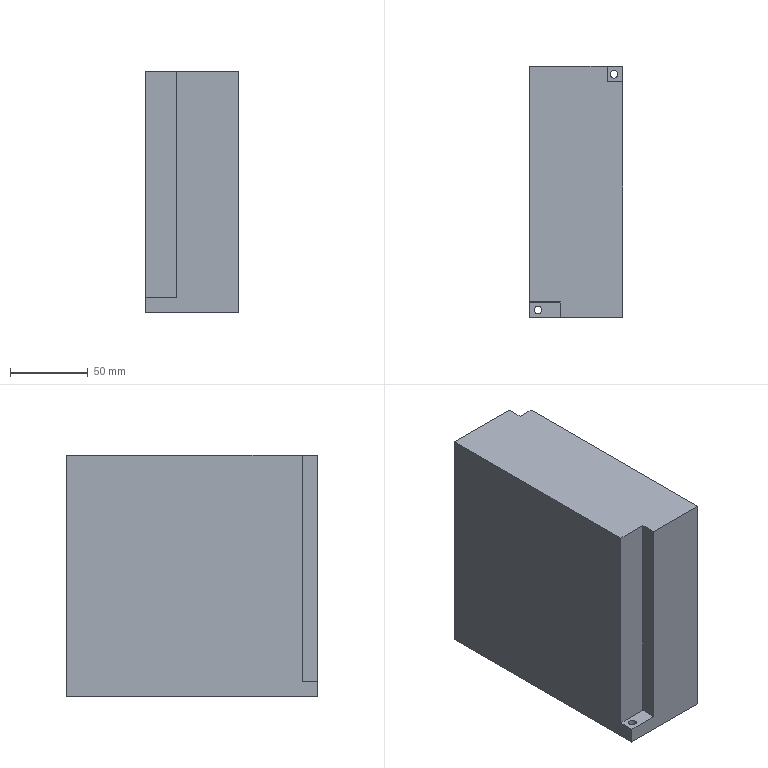Part | SolidWorks | features Cut 2, Extrusion 1 | 1 solid | 16 faces | box 60.2 x 162 x 155.9 mm | volume 1476236 mm3 | plane 12 | cylinder 4 | commonest cylinder face diameters 5 x4
STEP:
#1=CARTESIAN_POINT('',(-27.,-76.,0.));
#2=VERTEX_POINT('',#1);
#3=CARTESIAN_POINT('',(-22.,-76.,0.));
#4=VERTEX_POINT('',#3);
#5=CARTESIAN_POINT('',(-24.5,-76.,0.));
#6=DIRECTION('',(0.,0.,1.));
#7=DIRECTION('',(1.,0.,0.));
#8=AXIS2_PLACEMENT_3D('',#5,#6,#7);
#9=CIRCLE('',#8,2.5);
#10=EDGE_CURVE('',#2,#4,#9,.T.);
#11=ORIENTED_EDGE('',*,*,#10,.F.);
#12=CARTESIAN_POINT('',(-27.,-76.,10.));
#13=VERTEX_POINT('',#12);
#14=CARTESIAN_POINT('',(-27.,-76.,0.));
#15=DIRECTION('',(0.,0.,1.));
#16=VECTOR('',#15,1000.);
#17=LINE('',#14,#16);
#18=EDGE_CURVE('',#2,#13,#17,.T.);
#19=ORIENTED_EDGE('',*,*,#18,.T.);
#20=CARTESIAN_POINT('',(-22.,-76.,10.));
#21=VERTEX_POINT('',#20);
#22=CARTESIAN_POINT('',(-24.5,-76.,10.));
#23=DIRECTION('',(0.,0.,-1.));
#24=DIRECTION('',(-1.,0.,0.));
#25=AXIS2_PLACEMENT_3D('',#22,#23,#24);
#26=CIRCLE('',#25,2.5);
#27=EDGE_CURVE('',#21,#13,#26,.T.);
#28=ORIENTED_EDGE('',*,*,#27,.F.);
#29=CARTESIAN_POINT('',(-22.,-76.,0.));
#30=DIRECTION('',(0.,0.,1.));
#31=VECTOR('',#30,1000.);
#32=LINE('',#29,#31);
#33=EDGE_CURVE('',#4,#21,#32,.T.);
#34=ORIENTED_EDGE('',*,*,#33,.F.);
#35=EDGE_LOOP('',(#11,#19,#28,#34));
#36=FACE_OUTER_BOUND('',#35,.T.);
#37=CARTESIAN_POINT('',(-24.5,-76.,0.));
#38=DIRECTION('',(0.,0.,1.));
#39=DIRECTION('',(1.,0.,0.));
#40=AXIS2_PLACEMENT_3D('',#37,#38,#39);
#41=CYLINDRICAL_SURFACE('',#40,2.5);
#42=ADVANCED_FACE('',(#36),#41,.F.);
#43=CARTESIAN_POINT('',(22.,76.,0.));
#44=VERTEX_POINT('',#43);
#45=CARTESIAN_POINT('',(27.,76.,0.));
#46=VERTEX_POINT('',#45);
#47=CARTESIAN_POINT('',(24.5,76.,0.));
#48=DIRECTION('',(0.,0.,1.));
#49=DIRECTION('',(1.,0.,0.));
#50=AXIS2_PLACEMENT_3D('',#47,#48,#49);
#51=CIRCLE('',#50,2.5);
#52=EDGE_CURVE('',#44,#46,#51,.T.);
#53=ORIENTED_EDGE('',*,*,#52,.F.);
#54=CARTESIAN_POINT('',(22.,76.,10.));
#55=VERTEX_POINT('',#54);
#56=CARTESIAN_POINT('',(22.,76.,0.));
#57=DIRECTION('',(0.,0.,1.));
#58=VECTOR('',#57,1000.);
#59=LINE('',#56,#58);
#60=EDGE_CURVE('',#44,#55,#59,.T.);
#61=ORIENTED_EDGE('',*,*,#60,.T.);
#62=CARTESIAN_POINT('',(27.,76.,10.));
#63=VERTEX_POINT('',#62);
#64=CARTESIAN_POINT('',(24.5,76.,10.));
#65=DIRECTION('',(0.,0.,-1.));
#66=DIRECTION('',(-1.,0.,0.));
#67=AXIS2_PLACEMENT_3D('',#64,#65,#66);
#68=CIRCLE('',#67,2.5);
#69=EDGE_CURVE('',#63,#55,#68,.T.);
#70=ORIENTED_EDGE('',*,*,#69,.F.);
#71=CARTESIAN_POINT('',(27.,76.,0.));
#72=DIRECTION('',(0.,0.,1.));
#73=VECTOR('',#72,1000.);
#74=LINE('',#71,#73);
#75=EDGE_CURVE('',#46,#63,#74,.T.);
#76=ORIENTED_EDGE('',*,*,#75,.F.);
#77=EDGE_LOOP('',(#53,#61,#70,#76));
#78=FACE_OUTER_BOUND('',#77,.T.);
#79=CARTESIAN_POINT('',(24.5,76.,0.));
#80=DIRECTION('',(0.,0.,1.));
#81=DIRECTION('',(1.,0.,0.));
#82=AXIS2_PLACEMENT_3D('',#79,#80,#81);
#83=CYLINDRICAL_SURFACE('',#82,2.5);
#84=ADVANCED_FACE('',(#78),#83,.F.);
#85=CARTESIAN_POINT('',(-30.1,-71.,10.));
#86=VERTEX_POINT('',#85);
#87=CARTESIAN_POINT('',(-30.1,-81.,10.));
#88=VERTEX_POINT('',#87);
#89=CARTESIAN_POINT('',(-30.1,-81.,10.));
#90=DIRECTION('',(0.,-1.,0.));
#91=VECTOR('',#90,1000.);
#92=LINE('',#89,#91);
#93=EDGE_CURVE('',#86,#88,#92,.T.);
#94=ORIENTED_EDGE('',*,*,#93,.F.);
#95=CARTESIAN_POINT('',(-30.1,-71.,155.9));
#96=VERTEX_POINT('',#95);
#97=CARTESIAN_POINT('',(-30.1,-71.,10.));
#98=DIRECTION('',(0.,0.,1.));
#99=VECTOR('',#98,1000.);
#100=LINE('',#97,#99);
#101=EDGE_CURVE('',#86,#96,#100,.T.);
#102=ORIENTED_EDGE('',*,*,#101,.T.);
#103=CARTESIAN_POINT('',(-30.1,81.,155.9));
#104=VERTEX_POINT('',#103);
#105=CARTESIAN_POINT('',(-30.1,81.,155.9));
#106=DIRECTION('',(0.,-1.,0.));
#107=VECTOR('',#106,1000.);
#108=LINE('',#105,#107);
#109=EDGE_CURVE('',#104,#96,#108,.T.);
#110=ORIENTED_EDGE('',*,*,#109,.F.);
#111=CARTESIAN_POINT('',(-30.1,81.,0.));
#112=VERTEX_POINT('',#111);
#113=CARTESIAN_POINT('',(-30.1,81.,155.9));
#114=DIRECTION('',(0.,0.,-1.));
#115=VECTOR('',#114,1000.);
#116=LINE('',#113,#115);
#117=EDGE_CURVE('',#104,#112,#116,.T.);
#118=ORIENTED_EDGE('',*,*,#117,.T.);
#119=CARTESIAN_POINT('',(-30.1,-81.,0.));
#120=VERTEX_POINT('',#119);
#121=CARTESIAN_POINT('',(-30.1,81.,0.));
#122=DIRECTION('',(0.,-1.,0.));
#123=VECTOR('',#122,1000.);
#124=LINE('',#121,#123);
#125=EDGE_CURVE('',#112,#120,#124,.T.);
#126=ORIENTED_EDGE('',*,*,#125,.T.);
#127=CARTESIAN_POINT('',(-30.1,-81.,155.9));
#128=DIRECTION('',(0.,0.,-1.));
#129=VECTOR('',#128,1000.);
#130=LINE('',#127,#129);
#131=EDGE_CURVE('',#88,#120,#130,.T.);
#132=ORIENTED_EDGE('',*,*,#131,.F.);
#133=EDGE_LOOP('',(#94,#102,#110,#118,#126,#132));
#134=FACE_OUTER_BOUND('',#133,.T.);
#135=CARTESIAN_POINT('',(-30.1,81.,155.9));
#136=DIRECTION('',(1.,0.,0.));
#137=DIRECTION('',(0.,1.,0.));
#138=AXIS2_PLACEMENT_3D('',#135,#136,#137);
#139=PLANE('',#138);
#140=ADVANCED_FACE('',(#134),#139,.F.);
#141=CARTESIAN_POINT('',(-10.1,-81.,155.9));
#142=VERTEX_POINT('',#141);
#143=CARTESIAN_POINT('',(30.1,-81.,155.9));
#144=VERTEX_POINT('',#143);
#145=CARTESIAN_POINT('',(-30.1,-81.,155.9));
#146=DIRECTION('',(1.,0.,0.));
#147=VECTOR('',#146,1000.);
#148=LINE('',#145,#147);
#149=EDGE_CURVE('',#142,#144,#148,.T.);
#150=ORIENTED_EDGE('',*,*,#149,.F.);
#151=CARTESIAN_POINT('',(-10.1,-81.,10.));
#152=VERTEX_POINT('',#151);
#153=CARTESIAN_POINT('',(-10.1,-81.,10.));
#154=DIRECTION('',(0.,0.,1.));
#155=VECTOR('',#154,1000.);
#156=LINE('',#153,#155);
#157=EDGE_CURVE('',#152,#142,#156,.T.);
#158=ORIENTED_EDGE('',*,*,#157,.F.);
#159=CARTESIAN_POINT('',(-30.1,-81.,10.));
#160=DIRECTION('',(1.,0.,0.));
#161=VECTOR('',#160,1000.);
#162=LINE('',#159,#161);
#163=EDGE_CURVE('',#88,#152,#162,.T.);
#164=ORIENTED_EDGE('',*,*,#163,.F.);
#165=ORIENTED_EDGE('',*,*,#131,.T.);
#166=CARTESIAN_POINT('',(30.1,-81.,0.));
#167=VERTEX_POINT('',#166);
#168=CARTESIAN_POINT('',(-30.1,-81.,0.));
#169=DIRECTION('',(1.,0.,0.));
#170=VECTOR('',#169,1000.);
#171=LINE('',#168,#170);
#172=EDGE_CURVE('',#120,#167,#171,.T.);
#173=ORIENTED_EDGE('',*,*,#172,.T.);
#174=CARTESIAN_POINT('',(30.1,-81.,155.9));
#175=DIRECTION('',(0.,0.,-1.));
#176=VECTOR('',#175,1000.);
#177=LINE('',#174,#176);
#178=EDGE_CURVE('',#144,#167,#177,.T.);
#179=ORIENTED_EDGE('',*,*,#178,.F.);
#180=EDGE_LOOP('',(#150,#158,#164,#165,#173,#179));
#181=FACE_OUTER_BOUND('',#180,.T.);
#182=CARTESIAN_POINT('',(-30.1,-81.,155.9));
#183=DIRECTION('',(0.,1.,0.));
#184=DIRECTION('',(0.,0.,1.));
#185=AXIS2_PLACEMENT_3D('',#182,#183,#184);
#186=PLANE('',#185);
#187=ADVANCED_FACE('',(#181),#186,.F.);
#188=CARTESIAN_POINT('',(30.1,71.,10.));
#189=VERTEX_POINT('',#188);
#190=CARTESIAN_POINT('',(30.1,81.,10.));
#191=VERTEX_POINT('',#190);
#192=CARTESIAN_POINT('',(30.1,81.,10.));
#193=DIRECTION('',(0.,1.,0.));
#194=VECTOR('',#193,1000.);
#195=LINE('',#192,#194);
#196=EDGE_CURVE('',#189,#191,#195,.T.);
#197=ORIENTED_EDGE('',*,*,#196,.F.);
#198=CARTESIAN_POINT('',(30.1,71.,155.9));
#199=VERTEX_POINT('',#198);
#200=CARTESIAN_POINT('',(30.1,71.,10.));
#201=DIRECTION('',(0.,0.,1.));
#202=VECTOR('',#201,1000.);
#203=LINE('',#200,#202);
#204=EDGE_CURVE('',#189,#199,#203,.T.);
#205=ORIENTED_EDGE('',*,*,#204,.T.);
#206=CARTESIAN_POINT('',(30.1,81.,155.9));
#207=DIRECTION('',(0.,1.,0.));
#208=VECTOR('',#207,1000.);
#209=LINE('',#206,#208);
#210=EDGE_CURVE('',#144,#199,#209,.T.);
#211=ORIENTED_EDGE('',*,*,#210,.F.);
#212=ORIENTED_EDGE('',*,*,#178,.T.);
#213=CARTESIAN_POINT('',(30.1,81.,0.));
#214=VERTEX_POINT('',#213);
#215=CARTESIAN_POINT('',(30.1,81.,0.));
#216=DIRECTION('',(0.,1.,0.));
#217=VECTOR('',#216,1000.);
#218=LINE('',#215,#217);
#219=EDGE_CURVE('',#167,#214,#218,.T.);
#220=ORIENTED_EDGE('',*,*,#219,.T.);
#221=CARTESIAN_POINT('',(30.1,81.,155.9));
#222=DIRECTION('',(0.,0.,-1.));
#223=VECTOR('',#222,1000.);
#224=LINE('',#221,#223);
#225=EDGE_CURVE('',#191,#214,#224,.T.);
#226=ORIENTED_EDGE('',*,*,#225,.F.);
#227=EDGE_LOOP('',(#197,#205,#211,#212,#220,#226));
#228=FACE_OUTER_BOUND('',#227,.T.);
#229=CARTESIAN_POINT('',(30.1,81.,155.9));
#230=DIRECTION('',(-1.,0.,0.));
#231=DIRECTION('',(0.,-1.,0.));
#232=AXIS2_PLACEMENT_3D('',#229,#230,#231);
#233=PLANE('',#232);
#234=ADVANCED_FACE('',(#228),#233,.F.);
#235=CARTESIAN_POINT('',(20.1,81.,155.9));
#236=VERTEX_POINT('',#235);
#237=CARTESIAN_POINT('',(-30.1,81.,155.9));
#238=DIRECTION('',(-1.,0.,0.));
#239=VECTOR('',#238,1000.);
#240=LINE('',#237,#239);
#241=EDGE_CURVE('',#236,#104,#240,.T.);
#242=ORIENTED_EDGE('',*,*,#241,.F.);
#243=CARTESIAN_POINT('',(20.1,81.,10.));
#244=VERTEX_POINT('',#243);
#245=CARTESIAN_POINT('',(20.1,81.,10.));
#246=DIRECTION('',(0.,0.,1.));
#247=VECTOR('',#246,1000.);
#248=LINE('',#245,#247);
#249=EDGE_CURVE('',#244,#236,#248,.T.);
#250=ORIENTED_EDGE('',*,*,#249,.F.);
#251=CARTESIAN_POINT('',(30.1,81.,10.));
#252=DIRECTION('',(-1.,0.,0.));
#253=VECTOR('',#252,1000.);
#254=LINE('',#251,#253);
#255=EDGE_CURVE('',#191,#244,#254,.T.);
#256=ORIENTED_EDGE('',*,*,#255,.F.);
#257=ORIENTED_EDGE('',*,*,#225,.T.);
#258=CARTESIAN_POINT('',(-30.1,81.,0.));
#259=DIRECTION('',(-1.,0.,0.));
#260=VECTOR('',#259,1000.);
#261=LINE('',#258,#260);
#262=EDGE_CURVE('',#214,#112,#261,.T.);
#263=ORIENTED_EDGE('',*,*,#262,.T.);
#264=ORIENTED_EDGE('',*,*,#117,.F.);
#265=EDGE_LOOP('',(#242,#250,#256,#257,#263,#264));
#266=FACE_OUTER_BOUND('',#265,.T.);
#267=CARTESIAN_POINT('',(-30.1,81.,155.9));
#268=DIRECTION('',(0.,-1.,0.));
#269=DIRECTION('',(0.,0.,-1.));
#270=AXIS2_PLACEMENT_3D('',#267,#268,#269);
#271=PLANE('',#270);
#272=ADVANCED_FACE('',(#266),#271,.F.);
#273=CARTESIAN_POINT('',(20.1,71.,155.9));
#274=VERTEX_POINT('',#273);
#275=CARTESIAN_POINT('',(30.1,71.,155.9));
#276=DIRECTION('',(1.,0.,0.));
#277=VECTOR('',#276,1000.);
#278=LINE('',#275,#277);
#279=EDGE_CURVE('',#274,#199,#278,.T.);
#280=ORIENTED_EDGE('',*,*,#279,.F.);
#281=CARTESIAN_POINT('',(20.1,81.,155.9));
#282=DIRECTION('',(0.,-1.,0.));
#283=VECTOR('',#282,1000.);
#284=LINE('',#281,#283);
#285=EDGE_CURVE('',#236,#274,#284,.T.);
#286=ORIENTED_EDGE('',*,*,#285,.F.);
#287=ORIENTED_EDGE('',*,*,#241,.T.);
#288=ORIENTED_EDGE('',*,*,#109,.T.);
#289=CARTESIAN_POINT('',(-10.1,-71.,155.9));
#290=VERTEX_POINT('',#289);
#291=CARTESIAN_POINT('',(-30.1,-71.,155.9));
#292=DIRECTION('',(-1.,0.,0.));
#293=VECTOR('',#292,1000.);
#294=LINE('',#291,#293);
#295=EDGE_CURVE('',#290,#96,#294,.T.);
#296=ORIENTED_EDGE('',*,*,#295,.F.);
#297=CARTESIAN_POINT('',(-10.1,-81.,155.9));
#298=DIRECTION('',(0.,1.,0.));
#299=VECTOR('',#298,1000.);
#300=LINE('',#297,#299);
#301=EDGE_CURVE('',#142,#290,#300,.T.);
#302=ORIENTED_EDGE('',*,*,#301,.F.);
#303=ORIENTED_EDGE('',*,*,#149,.T.);
#304=ORIENTED_EDGE('',*,*,#210,.T.);
#305=EDGE_LOOP('',(#280,#286,#287,#288,#296,#302,#303,#304));
#306=FACE_OUTER_BOUND('',#305,.T.);
#307=CARTESIAN_POINT('',(-30.1,-81.,155.9));
#308=DIRECTION('',(0.,0.,1.));
#309=DIRECTION('',(1.,0.,0.));
#310=AXIS2_PLACEMENT_3D('',#307,#308,#309);
#311=PLANE('',#310);
#312=ADVANCED_FACE('',(#306),#311,.T.);
#313=CARTESIAN_POINT('',(-24.5,-76.,0.));
#314=DIRECTION('',(0.,0.,1.));
#315=DIRECTION('',(1.,0.,0.));
#316=AXIS2_PLACEMENT_3D('',#313,#314,#315);
#317=CIRCLE('',#316,2.5);
#318=EDGE_CURVE('',#4,#2,#317,.T.);
#319=ORIENTED_EDGE('',*,*,#318,.T.);
#320=ORIENTED_EDGE('',*,*,#10,.T.);
#321=EDGE_LOOP('',(#319,#320));
#322=FACE_BOUND('',#321,.T.);
#323=CARTESIAN_POINT('',(24.5,76.,0.));
#324=DIRECTION('',(0.,0.,1.));
#325=DIRECTION('',(1.,0.,0.));
#326=AXIS2_PLACEMENT_3D('',#323,#324,#325);
#327=CIRCLE('',#326,2.5);
#328=EDGE_CURVE('',#46,#44,#327,.T.);
#329=ORIENTED_EDGE('',*,*,#328,.T.);
#330=ORIENTED_EDGE('',*,*,#52,.T.);
#331=EDGE_LOOP('',(#329,#330));
#332=FACE_BOUND('',#331,.T.);
#333=ORIENTED_EDGE('',*,*,#125,.F.);
#334=ORIENTED_EDGE('',*,*,#262,.F.);
#335=ORIENTED_EDGE('',*,*,#219,.F.);
#336=ORIENTED_EDGE('',*,*,#172,.F.);
#337=EDGE_LOOP('',(#333,#334,#335,#336));
#338=FACE_OUTER_BOUND('',#337,.T.);
#339=CARTESIAN_POINT('',(-30.1,-81.,0.));
#340=DIRECTION('',(0.,0.,1.));
#341=DIRECTION('',(1.,0.,0.));
#342=AXIS2_PLACEMENT_3D('',#339,#340,#341);
#343=PLANE('',#342);
#344=ADVANCED_FACE('',(#322,#332,#338),#343,.F.);
#345=ORIENTED_EDGE('',*,*,#295,.T.);
#346=ORIENTED_EDGE('',*,*,#101,.F.);
#347=CARTESIAN_POINT('',(-10.1,-71.,10.));
#348=VERTEX_POINT('',#347);
#349=CARTESIAN_POINT('',(-30.1,-71.,10.));
#350=DIRECTION('',(-1.,0.,0.));
#351=VECTOR('',#350,1000.);
#352=LINE('',#349,#351);
#353=EDGE_CURVE('',#348,#86,#352,.T.);
#354=ORIENTED_EDGE('',*,*,#353,.F.);
#355=CARTESIAN_POINT('',(-10.1,-71.,10.));
#356=DIRECTION('',(0.,0.,1.));
#357=VECTOR('',#356,1000.);
#358=LINE('',#355,#357);
#359=EDGE_CURVE('',#348,#290,#358,.T.);
#360=ORIENTED_EDGE('',*,*,#359,.T.);
#361=EDGE_LOOP('',(#345,#346,#354,#360));
#362=FACE_OUTER_BOUND('',#361,.T.);
#363=CARTESIAN_POINT('',(-30.1,-71.,10.));
#364=DIRECTION('',(0.,1.,0.));
#365=DIRECTION('',(0.,0.,1.));
#366=AXIS2_PLACEMENT_3D('',#363,#364,#365);
#367=PLANE('',#366);
#368=ADVANCED_FACE('',(#362),#367,.F.);
#369=ORIENTED_EDGE('',*,*,#301,.T.);
#370=ORIENTED_EDGE('',*,*,#359,.F.);
#371=CARTESIAN_POINT('',(-10.1,-81.,10.));
#372=DIRECTION('',(0.,1.,0.));
#373=VECTOR('',#372,1000.);
#374=LINE('',#371,#373);
#375=EDGE_CURVE('',#152,#348,#374,.T.);
#376=ORIENTED_EDGE('',*,*,#375,.F.);
#377=ORIENTED_EDGE('',*,*,#157,.T.);
#378=EDGE_LOOP('',(#369,#370,#376,#377));
#379=FACE_OUTER_BOUND('',#378,.T.);
#380=CARTESIAN_POINT('',(-10.1,-81.,10.));
#381=DIRECTION('',(1.,0.,0.));
#382=DIRECTION('',(0.,0.,-1.));
#383=AXIS2_PLACEMENT_3D('',#380,#381,#382);
#384=PLANE('',#383);
#385=ADVANCED_FACE('',(#379),#384,.F.);
#386=ORIENTED_EDGE('',*,*,#27,.T.);
#387=CARTESIAN_POINT('',(-24.5,-76.,10.));
#388=DIRECTION('',(0.,0.,-1.));
#389=DIRECTION('',(-1.,0.,0.));
#390=AXIS2_PLACEMENT_3D('',#387,#388,#389);
#391=CIRCLE('',#390,2.5);
#392=EDGE_CURVE('',#13,#21,#391,.T.);
#393=ORIENTED_EDGE('',*,*,#392,.T.);
#394=EDGE_LOOP('',(#386,#393));
#395=FACE_BOUND('',#394,.T.);
#396=ORIENTED_EDGE('',*,*,#93,.T.);
#397=ORIENTED_EDGE('',*,*,#163,.T.);
#398=ORIENTED_EDGE('',*,*,#375,.T.);
#399=ORIENTED_EDGE('',*,*,#353,.T.);
#400=EDGE_LOOP('',(#396,#397,#398,#399));
#401=FACE_OUTER_BOUND('',#400,.T.);
#402=CARTESIAN_POINT('',(-30.1,-71.,10.));
#403=DIRECTION('',(0.,0.,-1.));
#404=DIRECTION('',(-1.,0.,0.));
#405=AXIS2_PLACEMENT_3D('',#402,#403,#404);
#406=PLANE('',#405);
#407=ADVANCED_FACE('',(#395,#401),#406,.F.);
#408=ORIENTED_EDGE('',*,*,#279,.T.);
#409=ORIENTED_EDGE('',*,*,#204,.F.);
#410=CARTESIAN_POINT('',(20.1,71.,10.));
#411=VERTEX_POINT('',#410);
#412=CARTESIAN_POINT('',(30.1,71.,10.));
#413=DIRECTION('',(1.,0.,0.));
#414=VECTOR('',#413,1000.);
#415=LINE('',#412,#414);
#416=EDGE_CURVE('',#411,#189,#415,.T.);
#417=ORIENTED_EDGE('',*,*,#416,.F.);
#418=CARTESIAN_POINT('',(20.1,71.,10.));
#419=DIRECTION('',(0.,0.,1.));
#420=VECTOR('',#419,1000.);
#421=LINE('',#418,#420);
#422=EDGE_CURVE('',#411,#274,#421,.T.);
#423=ORIENTED_EDGE('',*,*,#422,.T.);
#424=EDGE_LOOP('',(#408,#409,#417,#423));
#425=FACE_OUTER_BOUND('',#424,.T.);
#426=CARTESIAN_POINT('',(30.1,71.,10.));
#427=DIRECTION('',(0.,-1.,0.));
#428=DIRECTION('',(0.,0.,-1.));
#429=AXIS2_PLACEMENT_3D('',#426,#427,#428);
#430=PLANE('',#429);
#431=ADVANCED_FACE('',(#425),#430,.F.);
#432=ORIENTED_EDGE('',*,*,#285,.T.);
#433=ORIENTED_EDGE('',*,*,#422,.F.);
#434=CARTESIAN_POINT('',(20.1,81.,10.));
#435=DIRECTION('',(0.,-1.,0.));
#436=VECTOR('',#435,1000.);
#437=LINE('',#434,#436);
#438=EDGE_CURVE('',#244,#411,#437,.T.);
#439=ORIENTED_EDGE('',*,*,#438,.F.);
#440=ORIENTED_EDGE('',*,*,#249,.T.);
#441=EDGE_LOOP('',(#432,#433,#439,#440));
#442=FACE_OUTER_BOUND('',#441,.T.);
#443=CARTESIAN_POINT('',(20.1,81.,10.));
#444=DIRECTION('',(-1.,0.,0.));
#445=DIRECTION('',(0.,0.,1.));
#446=AXIS2_PLACEMENT_3D('',#443,#444,#445);
#447=PLANE('',#446);
#448=ADVANCED_FACE('',(#442),#447,.F.);
#449=ORIENTED_EDGE('',*,*,#69,.T.);
#450=CARTESIAN_POINT('',(24.5,76.,10.));
#451=DIRECTION('',(0.,0.,-1.));
#452=DIRECTION('',(-1.,0.,0.));
#453=AXIS2_PLACEMENT_3D('',#450,#451,#452);
#454=CIRCLE('',#453,2.5);
#455=EDGE_CURVE('',#55,#63,#454,.T.);
#456=ORIENTED_EDGE('',*,*,#455,.T.);
#457=EDGE_LOOP('',(#449,#456));
#458=FACE_BOUND('',#457,.T.);
#459=ORIENTED_EDGE('',*,*,#196,.T.);
#460=ORIENTED_EDGE('',*,*,#255,.T.);
#461=ORIENTED_EDGE('',*,*,#438,.T.);
#462=ORIENTED_EDGE('',*,*,#416,.T.);
#463=EDGE_LOOP('',(#459,#460,#461,#462));
#464=FACE_OUTER_BOUND('',#463,.T.);
#465=CARTESIAN_POINT('',(30.1,71.,10.));
#466=DIRECTION('',(0.,0.,-1.));
#467=DIRECTION('',(-1.,0.,0.));
#468=AXIS2_PLACEMENT_3D('',#465,#466,#467);
#469=PLANE('',#468);
#470=ADVANCED_FACE('',(#458,#464),#469,.F.);
#471=ORIENTED_EDGE('',*,*,#60,.F.);
#472=ORIENTED_EDGE('',*,*,#328,.F.);
#473=ORIENTED_EDGE('',*,*,#75,.T.);
#474=ORIENTED_EDGE('',*,*,#455,.F.);
#475=EDGE_LOOP('',(#471,#472,#473,#474));
#476=FACE_OUTER_BOUND('',#475,.T.);
#477=CARTESIAN_POINT('',(24.5,76.,0.));
#478=DIRECTION('',(0.,0.,1.));
#479=DIRECTION('',(1.,0.,0.));
#480=AXIS2_PLACEMENT_3D('',#477,#478,#479);
#481=CYLINDRICAL_SURFACE('',#480,2.5);
#482=ADVANCED_FACE('',(#476),#481,.F.);
#483=ORIENTED_EDGE('',*,*,#18,.F.);
#484=ORIENTED_EDGE('',*,*,#318,.F.);
#485=ORIENTED_EDGE('',*,*,#33,.T.);
#486=ORIENTED_EDGE('',*,*,#392,.F.);
#487=EDGE_LOOP('',(#483,#484,#485,#486));
#488=FACE_OUTER_BOUND('',#487,.T.);
#489=CARTESIAN_POINT('',(-24.5,-76.,0.));
#490=DIRECTION('',(0.,0.,1.));
#491=DIRECTION('',(1.,0.,0.));
#492=AXIS2_PLACEMENT_3D('',#489,#490,#491);
#493=CYLINDRICAL_SURFACE('',#492,2.5);
#494=ADVANCED_FACE('',(#488),#493,.F.);
#495=CLOSED_SHELL('',(#42,#84,#140,#187,#234,#272,#312,#344,#368,#385,#407,#431,#448,#470,#482,#494));
#496=MANIFOLD_SOLID_BREP('',#495);
#497=CARTESIAN_POINT('',(0.,0.,0.));
#498=DIRECTION('',(0.,0.,1.));
#499=DIRECTION('',(1.,0.,0.));
#500=AXIS2_PLACEMENT_3D('',#497,#498,#499);
#501=(LENGTH_UNIT()NAMED_UNIT(*)SI_UNIT(.MILLI.,.METRE.));
#502=UNCERTAINTY_MEASURE_WITH_UNIT(LENGTH_MEASURE(0.00001),#501,'','');
#503=(NAMED_UNIT(*)PLANE_ANGLE_UNIT()SI_UNIT($,.RADIAN.));
#504=(NAMED_UNIT(*)SI_UNIT($,.STERADIAN.)SOLID_ANGLE_UNIT());
#505=(GEOMETRIC_REPRESENTATION_CONTEXT(3)GLOBAL_UNCERTAINTY_ASSIGNED_CONTEXT((#502))GLOBAL_UNIT_ASSIGNED_CONTEXT((#501,#503,#504))REPRESENTATION_CONTEXT('',''));
#506=ADVANCED_BREP_SHAPE_REPRESENTATION('',(#496,#500),#505);